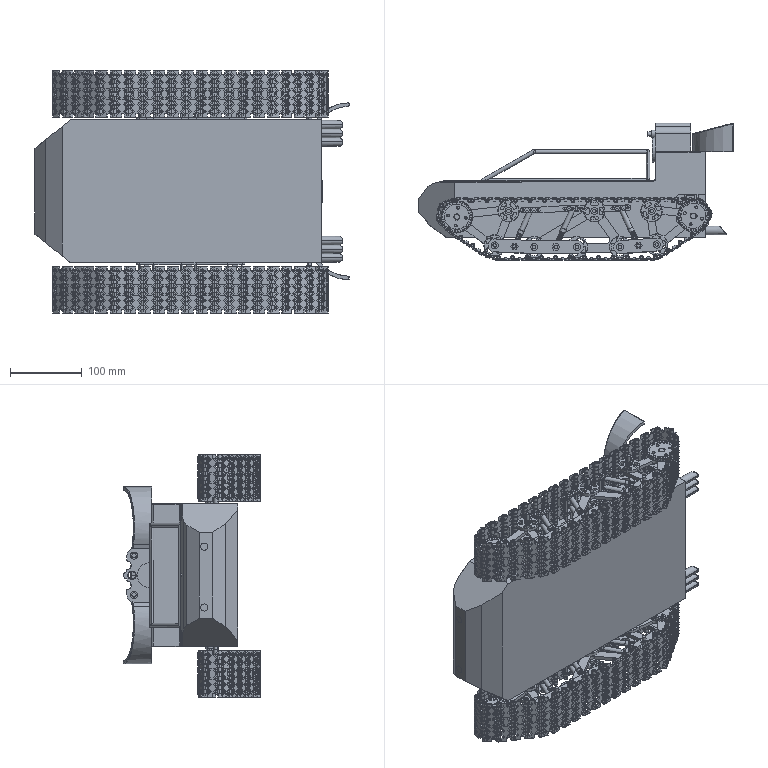Part | SolidWorks | features CompositeCurve 161, Cut 2 | 476 solids | 36775 faces | volume 5126066 mm3 | plane 25621 | cylinder 9856 | spline 594 | cone 400 | torus 300 | sphere 4 | commonest cylinder face diameters 5.8 x2706 3 x2133 1.032 x1312 4 x744 2 x529 5 x332